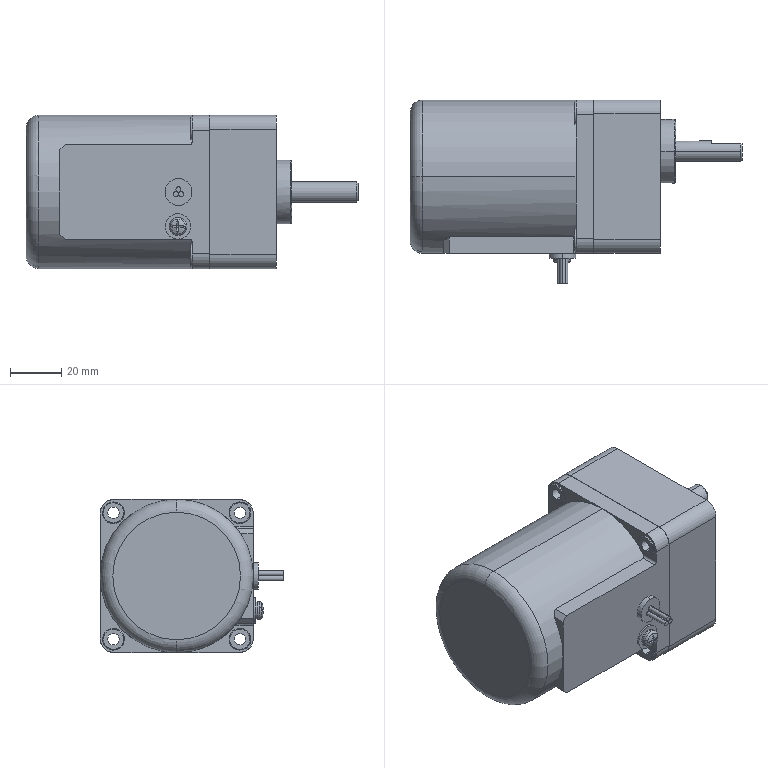Part | SolidWorks | features BaseBody 2 | 2 solids | 158 faces | box 130 x 72 x 60 mm | volume 275095 mm3 | plane 71 | cylinder 64 | torus 16 | sphere 4 | cone 3 | commonest cylinder face diameters 4.5 x16 2 x8 8.5 x8 4 x4 10.8 x4 11.5 x4